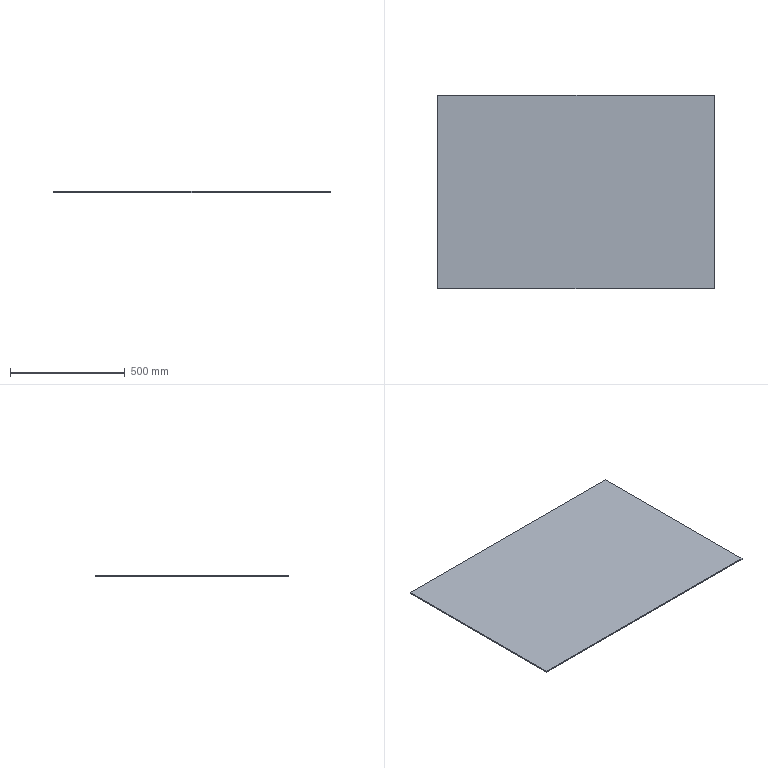Part | SolidWorks | features Extrusion 1, HoleWzd 1 | 1 solid | 6 faces | box 1206 x 842 x 5 mm | volume 5077260 mm3 | plane 6
STEP:
#1=CARTESIAN_POINT('',(603.,-421.,0.));
#2=VERTEX_POINT('',#1);
#3=CARTESIAN_POINT('',(603.,421.,0.));
#4=VERTEX_POINT('',#3);
#5=CARTESIAN_POINT('',(603.,421.,0.));
#6=DIRECTION('',(0.,1.,0.));
#7=VECTOR('',#6,1000.);
#8=LINE('',#5,#7);
#9=EDGE_CURVE('',#2,#4,#8,.T.);
#10=ORIENTED_EDGE('',*,*,#9,.T.);
#11=CARTESIAN_POINT('',(603.,421.,5.));
#12=VERTEX_POINT('',#11);
#13=CARTESIAN_POINT('',(603.,421.,5.));
#14=DIRECTION('',(0.,0.,-1.));
#15=VECTOR('',#14,1000.);
#16=LINE('',#13,#15);
#17=EDGE_CURVE('',#12,#4,#16,.T.);
#18=ORIENTED_EDGE('',*,*,#17,.F.);
#19=CARTESIAN_POINT('',(603.,-421.,5.));
#20=VERTEX_POINT('',#19);
#21=CARTESIAN_POINT('',(603.,421.,5.));
#22=DIRECTION('',(0.,1.,0.));
#23=VECTOR('',#22,1000.);
#24=LINE('',#21,#23);
#25=EDGE_CURVE('',#20,#12,#24,.T.);
#26=ORIENTED_EDGE('',*,*,#25,.F.);
#27=CARTESIAN_POINT('',(603.,-421.,5.));
#28=DIRECTION('',(0.,0.,-1.));
#29=VECTOR('',#28,1000.);
#30=LINE('',#27,#29);
#31=EDGE_CURVE('',#20,#2,#30,.T.);
#32=ORIENTED_EDGE('',*,*,#31,.T.);
#33=EDGE_LOOP('',(#10,#18,#26,#32));
#34=FACE_OUTER_BOUND('',#33,.T.);
#35=CARTESIAN_POINT('',(603.,421.,5.));
#36=DIRECTION('',(-1.,0.,0.));
#37=DIRECTION('',(0.,-1.,0.));
#38=AXIS2_PLACEMENT_3D('',#35,#36,#37);
#39=PLANE('',#38);
#40=ADVANCED_FACE('',(#34),#39,.F.);
#41=CARTESIAN_POINT('',(-603.,421.,0.));
#42=VERTEX_POINT('',#41);
#43=CARTESIAN_POINT('',(-603.,421.,0.));
#44=DIRECTION('',(-1.,0.,0.));
#45=VECTOR('',#44,1000.);
#46=LINE('',#43,#45);
#47=EDGE_CURVE('',#4,#42,#46,.T.);
#48=ORIENTED_EDGE('',*,*,#47,.T.);
#49=CARTESIAN_POINT('',(-603.,421.,5.));
#50=VERTEX_POINT('',#49);
#51=CARTESIAN_POINT('',(-603.,421.,5.));
#52=DIRECTION('',(0.,0.,-1.));
#53=VECTOR('',#52,1000.);
#54=LINE('',#51,#53);
#55=EDGE_CURVE('',#50,#42,#54,.T.);
#56=ORIENTED_EDGE('',*,*,#55,.F.);
#57=CARTESIAN_POINT('',(-603.,421.,5.));
#58=DIRECTION('',(-1.,0.,0.));
#59=VECTOR('',#58,1000.);
#60=LINE('',#57,#59);
#61=EDGE_CURVE('',#12,#50,#60,.T.);
#62=ORIENTED_EDGE('',*,*,#61,.F.);
#63=ORIENTED_EDGE('',*,*,#17,.T.);
#64=EDGE_LOOP('',(#48,#56,#62,#63));
#65=FACE_OUTER_BOUND('',#64,.T.);
#66=CARTESIAN_POINT('',(-603.,421.,5.));
#67=DIRECTION('',(0.,-1.,0.));
#68=DIRECTION('',(0.,0.,-1.));
#69=AXIS2_PLACEMENT_3D('',#66,#67,#68);
#70=PLANE('',#69);
#71=ADVANCED_FACE('',(#65),#70,.F.);
#72=CARTESIAN_POINT('',(-603.,-421.,0.));
#73=VERTEX_POINT('',#72);
#74=CARTESIAN_POINT('',(-603.,421.,0.));
#75=DIRECTION('',(0.,-1.,0.));
#76=VECTOR('',#75,1000.);
#77=LINE('',#74,#76);
#78=EDGE_CURVE('',#42,#73,#77,.T.);
#79=ORIENTED_EDGE('',*,*,#78,.T.);
#80=CARTESIAN_POINT('',(-603.,-421.,5.));
#81=VERTEX_POINT('',#80);
#82=CARTESIAN_POINT('',(-603.,-421.,5.));
#83=DIRECTION('',(0.,0.,-1.));
#84=VECTOR('',#83,1000.);
#85=LINE('',#82,#84);
#86=EDGE_CURVE('',#81,#73,#85,.T.);
#87=ORIENTED_EDGE('',*,*,#86,.F.);
#88=CARTESIAN_POINT('',(-603.,421.,5.));
#89=DIRECTION('',(0.,-1.,0.));
#90=VECTOR('',#89,1000.);
#91=LINE('',#88,#90);
#92=EDGE_CURVE('',#50,#81,#91,.T.);
#93=ORIENTED_EDGE('',*,*,#92,.F.);
#94=ORIENTED_EDGE('',*,*,#55,.T.);
#95=EDGE_LOOP('',(#79,#87,#93,#94));
#96=FACE_OUTER_BOUND('',#95,.T.);
#97=CARTESIAN_POINT('',(-603.,421.,5.));
#98=DIRECTION('',(1.,0.,0.));
#99=DIRECTION('',(0.,1.,0.));
#100=AXIS2_PLACEMENT_3D('',#97,#98,#99);
#101=PLANE('',#100);
#102=ADVANCED_FACE('',(#96),#101,.F.);
#103=CARTESIAN_POINT('',(-603.,-421.,0.));
#104=DIRECTION('',(1.,0.,0.));
#105=VECTOR('',#104,1000.);
#106=LINE('',#103,#105);
#107=EDGE_CURVE('',#73,#2,#106,.T.);
#108=ORIENTED_EDGE('',*,*,#107,.T.);
#109=ORIENTED_EDGE('',*,*,#31,.F.);
#110=CARTESIAN_POINT('',(-603.,-421.,5.));
#111=DIRECTION('',(1.,0.,0.));
#112=VECTOR('',#111,1000.);
#113=LINE('',#110,#112);
#114=EDGE_CURVE('',#81,#20,#113,.T.);
#115=ORIENTED_EDGE('',*,*,#114,.F.);
#116=ORIENTED_EDGE('',*,*,#86,.T.);
#117=EDGE_LOOP('',(#108,#109,#115,#116));
#118=FACE_OUTER_BOUND('',#117,.T.);
#119=CARTESIAN_POINT('',(-603.,-421.,5.));
#120=DIRECTION('',(0.,1.,0.));
#121=DIRECTION('',(0.,0.,1.));
#122=AXIS2_PLACEMENT_3D('',#119,#120,#121);
#123=PLANE('',#122);
#124=ADVANCED_FACE('',(#118),#123,.F.);
#125=ORIENTED_EDGE('',*,*,#25,.T.);
#126=ORIENTED_EDGE('',*,*,#61,.T.);
#127=ORIENTED_EDGE('',*,*,#92,.T.);
#128=ORIENTED_EDGE('',*,*,#114,.T.);
#129=EDGE_LOOP('',(#125,#126,#127,#128));
#130=FACE_OUTER_BOUND('',#129,.T.);
#131=CARTESIAN_POINT('',(0.,0.,5.));
#132=DIRECTION('',(0.,0.,1.));
#133=DIRECTION('',(1.,0.,0.));
#134=AXIS2_PLACEMENT_3D('',#131,#132,#133);
#135=PLANE('',#134);
#136=ADVANCED_FACE('',(#130),#135,.T.);
#137=ORIENTED_EDGE('',*,*,#9,.F.);
#138=ORIENTED_EDGE('',*,*,#107,.F.);
#139=ORIENTED_EDGE('',*,*,#78,.F.);
#140=ORIENTED_EDGE('',*,*,#47,.F.);
#141=EDGE_LOOP('',(#137,#138,#139,#140));
#142=FACE_OUTER_BOUND('',#141,.T.);
#143=CARTESIAN_POINT('',(0.,0.,0.));
#144=DIRECTION('',(0.,0.,1.));
#145=DIRECTION('',(1.,0.,0.));
#146=AXIS2_PLACEMENT_3D('',#143,#144,#145);
#147=PLANE('',#146);
#148=ADVANCED_FACE('',(#142),#147,.F.);
#149=CLOSED_SHELL('',(#40,#71,#102,#124,#136,#148));
#150=MANIFOLD_SOLID_BREP('',#149);
#151=CARTESIAN_POINT('',(0.,0.,0.));
#152=DIRECTION('',(0.,0.,1.));
#153=DIRECTION('',(1.,0.,0.));
#154=AXIS2_PLACEMENT_3D('',#151,#152,#153);
#155=(LENGTH_UNIT()NAMED_UNIT(*)SI_UNIT(.MILLI.,.METRE.));
#156=UNCERTAINTY_MEASURE_WITH_UNIT(LENGTH_MEASURE(0.00001),#155,'','');
#157=(NAMED_UNIT(*)PLANE_ANGLE_UNIT()SI_UNIT($,.RADIAN.));
#158=(NAMED_UNIT(*)SI_UNIT($,.STERADIAN.)SOLID_ANGLE_UNIT());
#159=(GEOMETRIC_REPRESENTATION_CONTEXT(3)GLOBAL_UNCERTAINTY_ASSIGNED_CONTEXT((#156))GLOBAL_UNIT_ASSIGNED_CONTEXT((#155,#157,#158))REPRESENTATION_CONTEXT('',''));
#160=ADVANCED_BREP_SHAPE_REPRESENTATION('',(#150,#154),#159);